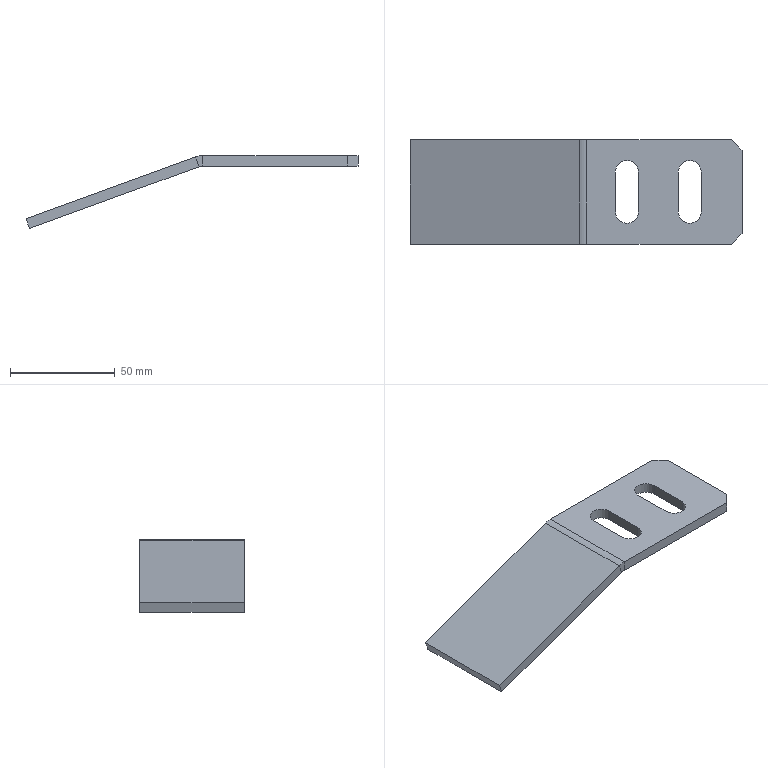Part | SolidWorks | features Chamfer 1, FlatPattern 1, ICE 1, SMBaseFlange 1, SheetMetal 1 | 1 solid | 24 faces | box 158.693 x 50 x 34.796 mm | volume 37608 mm3 | plane 18 | cylinder 6 | commonest cylinder face diameters 11 x4 10 x1 20 x1
STEP:
#1=CARTESIAN_POINT('',(-77.657,50.,-0.6031));
#2=VERTEX_POINT('',#1);
#3=CARTESIAN_POINT('',(-75.947,50.,-5.302));
#4=VERTEX_POINT('',#3);
#5=CARTESIAN_POINT('',(-77.657,50.,-0.6031));
#6=DIRECTION('',(0.342,0.,-0.9397));
#7=VECTOR('',#6,1000.);
#8=LINE('',#5,#7);
#9=EDGE_CURVE('',#2,#4,#8,.T.);
#10=ORIENTED_EDGE('',*,*,#9,.F.);
#11=CARTESIAN_POINT('',(-74.237,50.,0.));
#12=VERTEX_POINT('',#11);
#13=CARTESIAN_POINT('',(-74.237,50.,-10.));
#14=DIRECTION('',(0.,-1.,0.));
#15=DIRECTION('',(0.,0.,1.));
#16=AXIS2_PLACEMENT_3D('',#13,#14,#15);
#17=CIRCLE('',#16,10.);
#18=EDGE_CURVE('',#12,#2,#17,.T.);
#19=ORIENTED_EDGE('',*,*,#18,.F.);
#20=CARTESIAN_POINT('',(-74.237,50.,-5.));
#21=VERTEX_POINT('',#20);
#22=CARTESIAN_POINT('',(-74.237,50.,-5.));
#23=DIRECTION('',(0.,0.,1.));
#24=VECTOR('',#23,1000.);
#25=LINE('',#22,#24);
#26=EDGE_CURVE('',#21,#12,#25,.T.);
#27=ORIENTED_EDGE('',*,*,#26,.F.);
#28=CARTESIAN_POINT('',(-74.237,50.,-10.));
#29=DIRECTION('',(0.,-1.,0.));
#30=DIRECTION('',(1.,0.,0.));
#31=AXIS2_PLACEMENT_3D('',#28,#29,#30);
#32=CIRCLE('',#31,5.);
#33=EDGE_CURVE('',#21,#4,#32,.T.);
#34=ORIENTED_EDGE('',*,*,#33,.T.);
#35=EDGE_LOOP('',(#10,#19,#27,#34));
#36=FACE_OUTER_BOUND('',#35,.T.);
#37=CARTESIAN_POINT('',(-77.657,50.,-0.6031));
#38=DIRECTION('',(0.,1.,0.));
#39=DIRECTION('',(0.,0.,1.));
#40=AXIS2_PLACEMENT_3D('',#37,#38,#39);
#41=PLANE('',#40);
#42=ADVANCED_FACE('',(#36),#41,.T.);
#43=CARTESIAN_POINT('',(-158.693,50.,-30.098));
#44=VERTEX_POINT('',#43);
#45=CARTESIAN_POINT('',(-76.,50.,0.));
#46=DIRECTION('',(-0.9397,0.,-0.342));
#47=VECTOR('',#46,1000.);
#48=LINE('',#45,#47);
#49=EDGE_CURVE('',#2,#44,#48,.T.);
#50=ORIENTED_EDGE('',*,*,#49,.F.);
#51=ORIENTED_EDGE('',*,*,#9,.T.);
#52=CARTESIAN_POINT('',(-156.983,50.,-34.796));
#53=VERTEX_POINT('',#52);
#54=CARTESIAN_POINT('',(-74.29,50.,-4.698));
#55=DIRECTION('',(-0.9397,0.,-0.342));
#56=VECTOR('',#55,1000.);
#57=LINE('',#54,#56);
#58=EDGE_CURVE('',#4,#53,#57,.T.);
#59=ORIENTED_EDGE('',*,*,#58,.T.);
#60=CARTESIAN_POINT('',(-158.693,50.,-30.098));
#61=DIRECTION('',(0.342,0.,-0.9397));
#62=VECTOR('',#61,1000.);
#63=LINE('',#60,#62);
#64=EDGE_CURVE('',#44,#53,#63,.T.);
#65=ORIENTED_EDGE('',*,*,#64,.F.);
#66=EDGE_LOOP('',(#50,#51,#59,#65));
#67=FACE_OUTER_BOUND('',#66,.T.);
#68=CARTESIAN_POINT('',(-74.237,50.,-5.));
#69=DIRECTION('',(0.,1.,0.));
#70=DIRECTION('',(0.,0.,1.));
#71=AXIS2_PLACEMENT_3D('',#68,#69,#70);
#72=PLANE('',#71);
#73=ADVANCED_FACE('',(#67),#72,.T.);
#74=CARTESIAN_POINT('',(-74.237,0.,0.));
#75=VERTEX_POINT('',#74);
#76=CARTESIAN_POINT('',(-74.237,0.,-5.));
#77=VERTEX_POINT('',#76);
#78=CARTESIAN_POINT('',(-74.237,0.,0.));
#79=DIRECTION('',(0.,0.,-1.));
#80=VECTOR('',#79,1000.);
#81=LINE('',#78,#80);
#82=EDGE_CURVE('',#75,#77,#81,.T.);
#83=ORIENTED_EDGE('',*,*,#82,.F.);
#84=CARTESIAN_POINT('',(-77.657,0.,-0.6031));
#85=VERTEX_POINT('',#84);
#86=CARTESIAN_POINT('',(-74.237,0.,-10.));
#87=DIRECTION('',(0.,-1.,0.));
#88=DIRECTION('',(0.,0.,1.));
#89=AXIS2_PLACEMENT_3D('',#86,#87,#88);
#90=CIRCLE('',#89,10.);
#91=EDGE_CURVE('',#75,#85,#90,.T.);
#92=ORIENTED_EDGE('',*,*,#91,.T.);
#93=CARTESIAN_POINT('',(-75.947,0.,-5.302));
#94=VERTEX_POINT('',#93);
#95=CARTESIAN_POINT('',(-75.947,0.,-5.302));
#96=DIRECTION('',(-0.342,0.,0.9397));
#97=VECTOR('',#96,1000.);
#98=LINE('',#95,#97);
#99=EDGE_CURVE('',#94,#85,#98,.T.);
#100=ORIENTED_EDGE('',*,*,#99,.F.);
#101=CARTESIAN_POINT('',(-74.237,0.,-10.));
#102=DIRECTION('',(0.,-1.,0.));
#103=DIRECTION('',(1.,0.,0.));
#104=AXIS2_PLACEMENT_3D('',#101,#102,#103);
#105=CIRCLE('',#104,5.);
#106=EDGE_CURVE('',#77,#94,#105,.T.);
#107=ORIENTED_EDGE('',*,*,#106,.F.);
#108=EDGE_LOOP('',(#83,#92,#100,#107));
#109=FACE_OUTER_BOUND('',#108,.T.);
#110=CARTESIAN_POINT('',(-74.237,0.,0.));
#111=DIRECTION('',(0.,-1.,0.));
#112=DIRECTION('',(0.,0.,-1.));
#113=AXIS2_PLACEMENT_3D('',#110,#111,#112);
#114=PLANE('',#113);
#115=ADVANCED_FACE('',(#109),#114,.T.);
#116=CARTESIAN_POINT('',(-5.,0.,-5.));
#117=VERTEX_POINT('',#116);
#118=CARTESIAN_POINT('',(0.,0.,-5.));
#119=DIRECTION('',(-1.,0.,0.));
#120=VECTOR('',#119,1000.);
#121=LINE('',#118,#120);
#122=EDGE_CURVE('',#117,#77,#121,.T.);
#123=ORIENTED_EDGE('',*,*,#122,.F.);
#124=CARTESIAN_POINT('',(-5.,0.,0.));
#125=VERTEX_POINT('',#124);
#126=CARTESIAN_POINT('',(-5.,0.,-5.302));
#127=DIRECTION('',(0.,0.,1.));
#128=VECTOR('',#127,1000.);
#129=LINE('',#126,#128);
#130=EDGE_CURVE('',#117,#125,#129,.T.);
#131=ORIENTED_EDGE('',*,*,#130,.T.);
#132=CARTESIAN_POINT('',(0.,0.,0.));
#133=DIRECTION('',(-1.,0.,0.));
#134=VECTOR('',#133,1000.);
#135=LINE('',#132,#134);
#136=EDGE_CURVE('',#125,#75,#135,.T.);
#137=ORIENTED_EDGE('',*,*,#136,.T.);
#138=ORIENTED_EDGE('',*,*,#82,.T.);
#139=EDGE_LOOP('',(#123,#131,#137,#138));
#140=FACE_OUTER_BOUND('',#139,.T.);
#141=CARTESIAN_POINT('',(-75.947,0.,-5.302));
#142=DIRECTION('',(0.,-1.,0.));
#143=DIRECTION('',(0.,0.,-1.));
#144=AXIS2_PLACEMENT_3D('',#141,#142,#143);
#145=PLANE('',#144);
#146=ADVANCED_FACE('',(#140),#145,.T.);
#147=CARTESIAN_POINT('',(-156.983,0.,-34.796));
#148=VERTEX_POINT('',#147);
#149=CARTESIAN_POINT('',(-74.29,0.,-4.698));
#150=DIRECTION('',(-0.9397,0.,-0.342));
#151=VECTOR('',#150,1000.);
#152=LINE('',#149,#151);
#153=EDGE_CURVE('',#94,#148,#152,.T.);
#154=ORIENTED_EDGE('',*,*,#153,.T.);
#155=CARTESIAN_POINT('',(-156.983,50.,-34.796));
#156=DIRECTION('',(0.,-1.,0.));
#157=VECTOR('',#156,1000.);
#158=LINE('',#155,#157);
#159=EDGE_CURVE('',#53,#148,#158,.T.);
#160=ORIENTED_EDGE('',*,*,#159,.F.);
#161=ORIENTED_EDGE('',*,*,#58,.F.);
#162=CARTESIAN_POINT('',(-75.947,50.,-5.302));
#163=DIRECTION('',(0.,-1.,0.));
#164=VECTOR('',#163,1000.);
#165=LINE('',#162,#164);
#166=EDGE_CURVE('',#4,#94,#165,.T.);
#167=ORIENTED_EDGE('',*,*,#166,.T.);
#168=EDGE_LOOP('',(#154,#160,#161,#167));
#169=FACE_OUTER_BOUND('',#168,.T.);
#170=CARTESIAN_POINT('',(-74.29,50.,-4.698));
#171=DIRECTION('',(-0.342,0.,0.9397));
#172=DIRECTION('',(0.9397,0.,0.342));
#173=AXIS2_PLACEMENT_3D('',#170,#171,#172);
#174=PLANE('',#173);
#175=ADVANCED_FACE('',(#169),#174,.F.);
#176=CARTESIAN_POINT('',(-158.693,0.,-30.098));
#177=VERTEX_POINT('',#176);
#178=CARTESIAN_POINT('',(-158.693,0.,-30.098));
#179=DIRECTION('',(0.342,0.,-0.9397));
#180=VECTOR('',#179,1000.);
#181=LINE('',#178,#180);
#182=EDGE_CURVE('',#177,#148,#181,.T.);
#183=ORIENTED_EDGE('',*,*,#182,.F.);
#184=CARTESIAN_POINT('',(-158.693,50.,-30.098));
#185=DIRECTION('',(0.,-1.,0.));
#186=VECTOR('',#185,1000.);
#187=LINE('',#184,#186);
#188=EDGE_CURVE('',#44,#177,#187,.T.);
#189=ORIENTED_EDGE('',*,*,#188,.F.);
#190=ORIENTED_EDGE('',*,*,#64,.T.);
#191=ORIENTED_EDGE('',*,*,#159,.T.);
#192=EDGE_LOOP('',(#183,#189,#190,#191));
#193=FACE_OUTER_BOUND('',#192,.T.);
#194=CARTESIAN_POINT('',(-158.693,50.,-30.098));
#195=DIRECTION('',(-0.9397,0.,-0.342));
#196=DIRECTION('',(-0.342,0.,0.9397));
#197=AXIS2_PLACEMENT_3D('',#194,#195,#196);
#198=PLANE('',#197);
#199=ADVANCED_FACE('',(#193),#198,.T.);
#200=CARTESIAN_POINT('',(-76.,0.,0.));
#201=DIRECTION('',(-0.9397,0.,-0.342));
#202=VECTOR('',#201,1000.);
#203=LINE('',#200,#202);
#204=EDGE_CURVE('',#85,#177,#203,.T.);
#205=ORIENTED_EDGE('',*,*,#204,.F.);
#206=CARTESIAN_POINT('',(-77.657,50.,-0.6031));
#207=DIRECTION('',(0.,-1.,0.));
#208=VECTOR('',#207,1000.);
#209=LINE('',#206,#208);
#210=EDGE_CURVE('',#2,#85,#209,.T.);
#211=ORIENTED_EDGE('',*,*,#210,.F.);
#212=ORIENTED_EDGE('',*,*,#49,.T.);
#213=ORIENTED_EDGE('',*,*,#188,.T.);
#214=EDGE_LOOP('',(#205,#211,#212,#213));
#215=FACE_OUTER_BOUND('',#214,.T.);
#216=CARTESIAN_POINT('',(-76.,50.,0.));
#217=DIRECTION('',(-0.342,0.,0.9397));
#218=DIRECTION('',(0.9397,0.,0.342));
#219=AXIS2_PLACEMENT_3D('',#216,#217,#218);
#220=PLANE('',#219);
#221=ADVANCED_FACE('',(#215),#220,.T.);
#222=ORIENTED_EDGE('',*,*,#91,.F.);
#223=CARTESIAN_POINT('',(-74.237,50.,0.));
#224=DIRECTION('',(0.,-1.,0.));
#225=VECTOR('',#224,1000.);
#226=LINE('',#223,#225);
#227=EDGE_CURVE('',#12,#75,#226,.T.);
#228=ORIENTED_EDGE('',*,*,#227,.F.);
#229=ORIENTED_EDGE('',*,*,#18,.T.);
#230=ORIENTED_EDGE('',*,*,#210,.T.);
#231=EDGE_LOOP('',(#222,#228,#229,#230));
#232=FACE_OUTER_BOUND('',#231,.T.);
#233=CARTESIAN_POINT('',(-74.237,50.,-10.));
#234=DIRECTION('',(0.,-1.,0.));
#235=DIRECTION('',(0.,0.,-1.));
#236=AXIS2_PLACEMENT_3D('',#233,#234,#235);
#237=CYLINDRICAL_SURFACE('',#236,10.);
#238=ADVANCED_FACE('',(#232),#237,.T.);
#239=CARTESIAN_POINT('',(-19.5,34.5,0.));
#240=VERTEX_POINT('',#239);
#241=CARTESIAN_POINT('',(-30.5,34.5,0.));
#242=VERTEX_POINT('',#241);
#243=CARTESIAN_POINT('',(-25.,34.5,0.));
#244=DIRECTION('',(0.,0.,1.));
#245=DIRECTION('',(1.,0.,0.));
#246=AXIS2_PLACEMENT_3D('',#243,#244,#245);
#247=CIRCLE('',#246,5.5);
#248=EDGE_CURVE('',#240,#242,#247,.T.);
#249=ORIENTED_EDGE('',*,*,#248,.F.);
#250=CARTESIAN_POINT('',(-19.5,15.5,0.));
#251=VERTEX_POINT('',#250);
#252=CARTESIAN_POINT('',(-19.5,34.5,0.));
#253=DIRECTION('',(0.,1.,0.));
#254=VECTOR('',#253,1000.);
#255=LINE('',#252,#254);
#256=EDGE_CURVE('',#251,#240,#255,.T.);
#257=ORIENTED_EDGE('',*,*,#256,.F.);
#258=CARTESIAN_POINT('',(-30.5,15.5,0.));
#259=VERTEX_POINT('',#258);
#260=CARTESIAN_POINT('',(-25.,15.5,0.));
#261=DIRECTION('',(0.,0.,1.));
#262=DIRECTION('',(1.,0.,0.));
#263=AXIS2_PLACEMENT_3D('',#260,#261,#262);
#264=CIRCLE('',#263,5.5);
#265=EDGE_CURVE('',#259,#251,#264,.T.);
#266=ORIENTED_EDGE('',*,*,#265,.F.);
#267=CARTESIAN_POINT('',(-30.5,34.5,0.));
#268=DIRECTION('',(0.,-1.,0.));
#269=VECTOR('',#268,1000.);
#270=LINE('',#267,#269);
#271=EDGE_CURVE('',#242,#259,#270,.T.);
#272=ORIENTED_EDGE('',*,*,#271,.F.);
#273=EDGE_LOOP('',(#249,#257,#266,#272));
#274=FACE_BOUND('',#273,.T.);
#275=CARTESIAN_POINT('',(-49.5,34.5,0.));
#276=VERTEX_POINT('',#275);
#277=CARTESIAN_POINT('',(-60.5,34.5,0.));
#278=VERTEX_POINT('',#277);
#279=CARTESIAN_POINT('',(-55.,34.5,0.));
#280=DIRECTION('',(0.,0.,1.));
#281=DIRECTION('',(1.,0.,0.));
#282=AXIS2_PLACEMENT_3D('',#279,#280,#281);
#283=CIRCLE('',#282,5.5);
#284=EDGE_CURVE('',#276,#278,#283,.T.);
#285=ORIENTED_EDGE('',*,*,#284,.F.);
#286=CARTESIAN_POINT('',(-49.5,15.5,0.));
#287=VERTEX_POINT('',#286);
#288=CARTESIAN_POINT('',(-49.5,34.5,0.));
#289=DIRECTION('',(0.,1.,0.));
#290=VECTOR('',#289,1000.);
#291=LINE('',#288,#290);
#292=EDGE_CURVE('',#287,#276,#291,.T.);
#293=ORIENTED_EDGE('',*,*,#292,.F.);
#294=CARTESIAN_POINT('',(-60.5,15.5,0.));
#295=VERTEX_POINT('',#294);
#296=CARTESIAN_POINT('',(-55.,15.5,0.));
#297=DIRECTION('',(0.,0.,1.));
#298=DIRECTION('',(1.,0.,0.));
#299=AXIS2_PLACEMENT_3D('',#296,#297,#298);
#300=CIRCLE('',#299,5.5);
#301=EDGE_CURVE('',#295,#287,#300,.T.);
#302=ORIENTED_EDGE('',*,*,#301,.F.);
#303=CARTESIAN_POINT('',(-60.5,34.5,0.));
#304=DIRECTION('',(0.,-1.,0.));
#305=VECTOR('',#304,1000.);
#306=LINE('',#303,#305);
#307=EDGE_CURVE('',#278,#295,#306,.T.);
#308=ORIENTED_EDGE('',*,*,#307,.F.);
#309=EDGE_LOOP('',(#285,#293,#302,#308));
#310=FACE_BOUND('',#309,.T.);
#311=ORIENTED_EDGE('',*,*,#136,.F.);
#312=CARTESIAN_POINT('',(0.,5.,0.));
#313=VERTEX_POINT('',#312);
#314=CARTESIAN_POINT('',(22.5,27.5,0.));
#315=DIRECTION('',(0.7071,0.7071,0.));
#316=VECTOR('',#315,1000.);
#317=LINE('',#314,#316);
#318=EDGE_CURVE('',#125,#313,#317,.T.);
#319=ORIENTED_EDGE('',*,*,#318,.T.);
#320=CARTESIAN_POINT('',(0.,45.,0.));
#321=VERTEX_POINT('',#320);
#322=CARTESIAN_POINT('',(0.,50.,0.));
#323=DIRECTION('',(0.,-1.,0.));
#324=VECTOR('',#323,1000.);
#325=LINE('',#322,#324);
#326=EDGE_CURVE('',#321,#313,#325,.T.);
#327=ORIENTED_EDGE('',*,*,#326,.F.);
#328=CARTESIAN_POINT('',(-5.,50.,0.));
#329=VERTEX_POINT('',#328);
#330=CARTESIAN_POINT('',(-2.5,47.5,0.));
#331=DIRECTION('',(-0.7071,0.7071,0.));
#332=VECTOR('',#331,1000.);
#333=LINE('',#330,#332);
#334=EDGE_CURVE('',#321,#329,#333,.T.);
#335=ORIENTED_EDGE('',*,*,#334,.T.);
#336=CARTESIAN_POINT('',(0.,50.,0.));
#337=DIRECTION('',(-1.,0.,0.));
#338=VECTOR('',#337,1000.);
#339=LINE('',#336,#338);
#340=EDGE_CURVE('',#329,#12,#339,.T.);
#341=ORIENTED_EDGE('',*,*,#340,.T.);
#342=ORIENTED_EDGE('',*,*,#227,.T.);
#343=EDGE_LOOP('',(#311,#319,#327,#335,#341,#342));
#344=FACE_OUTER_BOUND('',#343,.T.);
#345=CARTESIAN_POINT('',(0.,50.,0.));
#346=DIRECTION('',(0.,0.,1.));
#347=DIRECTION('',(1.,0.,0.));
#348=AXIS2_PLACEMENT_3D('',#345,#346,#347);
#349=PLANE('',#348);
#350=ADVANCED_FACE('',(#274,#310,#344),#349,.T.);
#351=ORIENTED_EDGE('',*,*,#326,.T.);
#352=CARTESIAN_POINT('',(0.,5.,-5.));
#353=VERTEX_POINT('',#352);
#354=CARTESIAN_POINT('',(0.,5.,-5.));
#355=DIRECTION('',(0.,0.,-1.));
#356=VECTOR('',#355,1000.);
#357=LINE('',#354,#356);
#358=EDGE_CURVE('',#313,#353,#357,.T.);
#359=ORIENTED_EDGE('',*,*,#358,.T.);
#360=CARTESIAN_POINT('',(0.,45.,-5.));
#361=VERTEX_POINT('',#360);
#362=CARTESIAN_POINT('',(0.,50.,-5.));
#363=DIRECTION('',(0.,-1.,0.));
#364=VECTOR('',#363,1000.);
#365=LINE('',#362,#364);
#366=EDGE_CURVE('',#361,#353,#365,.T.);
#367=ORIENTED_EDGE('',*,*,#366,.F.);
#368=CARTESIAN_POINT('',(0.,45.,-5.));
#369=DIRECTION('',(0.,0.,1.));
#370=VECTOR('',#369,1000.);
#371=LINE('',#368,#370);
#372=EDGE_CURVE('',#361,#321,#371,.T.);
#373=ORIENTED_EDGE('',*,*,#372,.T.);
#374=EDGE_LOOP('',(#351,#359,#367,#373));
#375=FACE_OUTER_BOUND('',#374,.T.);
#376=CARTESIAN_POINT('',(0.,50.,-5.));
#377=DIRECTION('',(1.,0.,0.));
#378=DIRECTION('',(0.,0.,-1.));
#379=AXIS2_PLACEMENT_3D('',#376,#377,#378);
#380=PLANE('',#379);
#381=ADVANCED_FACE('',(#375),#380,.T.);
#382=CARTESIAN_POINT('',(-19.5,15.5,-5.));
#383=VERTEX_POINT('',#382);
#384=CARTESIAN_POINT('',(-19.5,34.5,-5.));
#385=VERTEX_POINT('',#384);
#386=CARTESIAN_POINT('',(-19.5,50.,-5.));
#387=DIRECTION('',(0.,1.,0.));
#388=VECTOR('',#387,1000.);
#389=LINE('',#386,#388);
#390=EDGE_CURVE('',#383,#385,#389,.T.);
#391=ORIENTED_EDGE('',*,*,#390,.T.);
#392=CARTESIAN_POINT('',(-30.5,34.5,-5.));
#393=VERTEX_POINT('',#392);
#394=CARTESIAN_POINT('',(-25.,34.5,-5.));
#395=DIRECTION('',(0.,0.,1.));
#396=DIRECTION('',(1.,0.,0.));
#397=AXIS2_PLACEMENT_3D('',#394,#395,#396);
#398=CIRCLE('',#397,5.5);
#399=EDGE_CURVE('',#385,#393,#398,.T.);
#400=ORIENTED_EDGE('',*,*,#399,.T.);
#401=CARTESIAN_POINT('',(-30.5,15.5,-5.));
#402=VERTEX_POINT('',#401);
#403=CARTESIAN_POINT('',(-30.5,50.,-5.));
#404=DIRECTION('',(0.,-1.,0.));
#405=VECTOR('',#404,1000.);
#406=LINE('',#403,#405);
#407=EDGE_CURVE('',#393,#402,#406,.T.);
#408=ORIENTED_EDGE('',*,*,#407,.T.);
#409=CARTESIAN_POINT('',(-25.,15.5,-5.));
#410=DIRECTION('',(0.,0.,1.));
#411=DIRECTION('',(1.,0.,0.));
#412=AXIS2_PLACEMENT_3D('',#409,#410,#411);
#413=CIRCLE('',#412,5.5);
#414=EDGE_CURVE('',#402,#383,#413,.T.);
#415=ORIENTED_EDGE('',*,*,#414,.T.);
#416=EDGE_LOOP('',(#391,#400,#408,#415));
#417=FACE_BOUND('',#416,.T.);
#418=CARTESIAN_POINT('',(-49.5,15.5,-5.));
#419=VERTEX_POINT('',#418);
#420=CARTESIAN_POINT('',(-49.5,34.5,-5.));
#421=VERTEX_POINT('',#420);
#422=CARTESIAN_POINT('',(-49.5,50.,-5.));
#423=DIRECTION('',(0.,1.,0.));
#424=VECTOR('',#423,1000.);
#425=LINE('',#422,#424);
#426=EDGE_CURVE('',#419,#421,#425,.T.);
#427=ORIENTED_EDGE('',*,*,#426,.T.);
#428=CARTESIAN_POINT('',(-60.5,34.5,-5.));
#429=VERTEX_POINT('',#428);
#430=CARTESIAN_POINT('',(-55.,34.5,-5.));
#431=DIRECTION('',(0.,0.,1.));
#432=DIRECTION('',(1.,0.,0.));
#433=AXIS2_PLACEMENT_3D('',#430,#431,#432);
#434=CIRCLE('',#433,5.5);
#435=EDGE_CURVE('',#421,#429,#434,.T.);
#436=ORIENTED_EDGE('',*,*,#435,.T.);
#437=CARTESIAN_POINT('',(-60.5,15.5,-5.));
#438=VERTEX_POINT('',#437);
#439=CARTESIAN_POINT('',(-60.5,50.,-5.));
#440=DIRECTION('',(0.,-1.,0.));
#441=VECTOR('',#440,1000.);
#442=LINE('',#439,#441);
#443=EDGE_CURVE('',#429,#438,#442,.T.);
#444=ORIENTED_EDGE('',*,*,#443,.T.);
#445=CARTESIAN_POINT('',(-55.,15.5,-5.));
#446=DIRECTION('',(0.,0.,1.));
#447=DIRECTION('',(1.,0.,0.));
#448=AXIS2_PLACEMENT_3D('',#445,#446,#447);
#449=CIRCLE('',#448,5.5);
#450=EDGE_CURVE('',#438,#419,#449,.T.);
#451=ORIENTED_EDGE('',*,*,#450,.T.);
#452=EDGE_LOOP('',(#427,#436,#444,#451));
#453=FACE_BOUND('',#452,.T.);
#454=ORIENTED_EDGE('',*,*,#366,.T.);
#455=CARTESIAN_POINT('',(-5.,0.,-5.));
#456=DIRECTION('',(-0.7071,-0.7071,0.));
#457=VECTOR('',#456,1000.);
#458=LINE('',#455,#457);
#459=EDGE_CURVE('',#353,#117,#458,.T.);
#460=ORIENTED_EDGE('',*,*,#459,.T.);
#461=ORIENTED_EDGE('',*,*,#122,.T.);
#462=CARTESIAN_POINT('',(-74.237,50.,-5.));
#463=DIRECTION('',(0.,-1.,0.));
#464=VECTOR('',#463,1000.);
#465=LINE('',#462,#464);
#466=EDGE_CURVE('',#21,#77,#465,.T.);
#467=ORIENTED_EDGE('',*,*,#466,.F.);
#468=CARTESIAN_POINT('',(-5.,50.,-5.));
#469=VERTEX_POINT('',#468);
#470=CARTESIAN_POINT('',(0.,50.,-5.));
#471=DIRECTION('',(-1.,0.,0.));
#472=VECTOR('',#471,1000.);
#473=LINE('',#470,#472);
#474=EDGE_CURVE('',#469,#21,#473,.T.);
#475=ORIENTED_EDGE('',*,*,#474,.F.);
#476=CARTESIAN_POINT('',(0.,45.,-5.));
#477=DIRECTION('',(0.7071,-0.7071,0.));
#478=VECTOR('',#477,1000.);
#479=LINE('',#476,#478);
#480=EDGE_CURVE('',#469,#361,#479,.T.);
#481=ORIENTED_EDGE('',*,*,#480,.T.);
#482=EDGE_LOOP('',(#454,#460,#461,#467,#475,#481));
#483=FACE_OUTER_BOUND('',#482,.T.);
#484=CARTESIAN_POINT('',(0.,50.,-5.));
#485=DIRECTION('',(0.,0.,1.));
#486=DIRECTION('',(1.,0.,0.));
#487=AXIS2_PLACEMENT_3D('',#484,#485,#486);
#488=PLANE('',#487);
#489=ADVANCED_FACE('',(#417,#453,#483),#488,.F.);
#490=ORIENTED_EDGE('',*,*,#106,.T.);
#491=ORIENTED_EDGE('',*,*,#166,.F.);
#492=ORIENTED_EDGE('',*,*,#33,.F.);
#493=ORIENTED_EDGE('',*,*,#466,.T.);
#494=EDGE_LOOP('',(#490,#491,#492,#493));
#495=FACE_OUTER_BOUND('',#494,.T.);
#496=CARTESIAN_POINT('',(-74.237,50.,-10.));
#497=DIRECTION('',(0.,-1.,0.));
#498=DIRECTION('',(0.,0.,-1.));
#499=AXIS2_PLACEMENT_3D('',#496,#497,#498);
#500=CYLINDRICAL_SURFACE('',#499,5.);
#501=ADVANCED_FACE('',(#495),#500,.F.);
#502=ORIENTED_EDGE('',*,*,#340,.F.);
#503=CARTESIAN_POINT('',(-5.,50.,-10.));
#504=DIRECTION('',(0.,0.,-1.));
#505=VECTOR('',#504,1000.);
#506=LINE('',#503,#505);
#507=EDGE_CURVE('',#329,#469,#506,.T.);
#508=ORIENTED_EDGE('',*,*,#507,.T.);
#509=ORIENTED_EDGE('',*,*,#474,.T.);
#510=ORIENTED_EDGE('',*,*,#26,.T.);
#511=EDGE_LOOP('',(#502,#508,#509,#510));
#512=FACE_OUTER_BOUND('',#511,.T.);
#513=CARTESIAN_POINT('',(-74.237,50.,-10.));
#514=DIRECTION('',(0.,1.,0.));
#515=DIRECTION('',(1.,0.,0.));
#516=AXIS2_PLACEMENT_3D('',#513,#514,#515);
#517=PLANE('',#516);
#518=ADVANCED_FACE('',(#512),#517,.T.);
#519=ORIENTED_EDGE('',*,*,#153,.F.);
#520=ORIENTED_EDGE('',*,*,#99,.T.);
#521=ORIENTED_EDGE('',*,*,#204,.T.);
#522=ORIENTED_EDGE('',*,*,#182,.T.);
#523=EDGE_LOOP('',(#519,#520,#521,#522));
#524=FACE_OUTER_BOUND('',#523,.T.);
#525=CARTESIAN_POINT('',(-74.237,0.,-10.));
#526=DIRECTION('',(0.,1.,0.));
#527=DIRECTION('',(1.,0.,0.));
#528=AXIS2_PLACEMENT_3D('',#525,#526,#527);
#529=PLANE('',#528);
#530=ADVANCED_FACE('',(#524),#529,.F.);
#531=CARTESIAN_POINT('',(-49.5,34.5,-10.));
#532=DIRECTION('',(0.,0.,1.));
#533=VECTOR('',#532,1000.);
#534=LINE('',#531,#533);
#535=EDGE_CURVE('',#421,#276,#534,.T.);
#536=ORIENTED_EDGE('',*,*,#535,.T.);
#537=ORIENTED_EDGE('',*,*,#284,.T.);
#538=CARTESIAN_POINT('',(-60.5,34.5,-10.));
#539=DIRECTION('',(0.,0.,1.));
#540=VECTOR('',#539,1000.);
#541=LINE('',#538,#540);
#542=EDGE_CURVE('',#429,#278,#541,.T.);
#543=ORIENTED_EDGE('',*,*,#542,.F.);
#544=ORIENTED_EDGE('',*,*,#435,.F.);
#545=EDGE_LOOP('',(#536,#537,#543,#544));
#546=FACE_OUTER_BOUND('',#545,.T.);
#547=CARTESIAN_POINT('',(-55.,34.5,-10.));
#548=DIRECTION('',(0.,0.,1.));
#549=DIRECTION('',(1.,0.,0.));
#550=AXIS2_PLACEMENT_3D('',#547,#548,#549);
#551=CYLINDRICAL_SURFACE('',#550,5.5);
#552=ADVANCED_FACE('',(#546),#551,.F.);
#553=CARTESIAN_POINT('',(-49.5,15.5,-10.));
#554=DIRECTION('',(0.,0.,1.));
#555=VECTOR('',#554,1000.);
#556=LINE('',#553,#555);
#557=EDGE_CURVE('',#419,#287,#556,.T.);
#558=ORIENTED_EDGE('',*,*,#557,.T.);
#559=ORIENTED_EDGE('',*,*,#292,.T.);
#560=ORIENTED_EDGE('',*,*,#535,.F.);
#561=ORIENTED_EDGE('',*,*,#426,.F.);
#562=EDGE_LOOP('',(#558,#559,#560,#561));
#563=FACE_OUTER_BOUND('',#562,.T.);
#564=CARTESIAN_POINT('',(-49.5,34.5,-10.));
#565=DIRECTION('',(1.,0.,0.));
#566=DIRECTION('',(0.,0.,-1.));
#567=AXIS2_PLACEMENT_3D('',#564,#565,#566);
#568=PLANE('',#567);
#569=ADVANCED_FACE('',(#563),#568,.F.);
#570=CARTESIAN_POINT('',(-60.5,15.5,-10.));
#571=DIRECTION('',(0.,0.,1.));
#572=VECTOR('',#571,1000.);
#573=LINE('',#570,#572);
#574=EDGE_CURVE('',#438,#295,#573,.T.);
#575=ORIENTED_EDGE('',*,*,#574,.T.);
#576=ORIENTED_EDGE('',*,*,#301,.T.);
#577=ORIENTED_EDGE('',*,*,#557,.F.);
#578=ORIENTED_EDGE('',*,*,#450,.F.);
#579=EDGE_LOOP('',(#575,#576,#577,#578));
#580=FACE_OUTER_BOUND('',#579,.T.);
#581=CARTESIAN_POINT('',(-55.,15.5,-10.));
#582=DIRECTION('',(0.,0.,1.));
#583=DIRECTION('',(1.,0.,0.));
#584=AXIS2_PLACEMENT_3D('',#581,#582,#583);
#585=CYLINDRICAL_SURFACE('',#584,5.5);
#586=ADVANCED_FACE('',(#580),#585,.F.);
#587=ORIENTED_EDGE('',*,*,#542,.T.);
#588=ORIENTED_EDGE('',*,*,#307,.T.);
#589=ORIENTED_EDGE('',*,*,#574,.F.);
#590=ORIENTED_EDGE('',*,*,#443,.F.);
#591=EDGE_LOOP('',(#587,#588,#589,#590));
#592=FACE_OUTER_BOUND('',#591,.T.);
#593=CARTESIAN_POINT('',(-60.5,34.5,-10.));
#594=DIRECTION('',(-1.,0.,0.));
#595=DIRECTION('',(0.,0.,1.));
#596=AXIS2_PLACEMENT_3D('',#593,#594,#595);
#597=PLANE('',#596);
#598=ADVANCED_FACE('',(#592),#597,.F.);
#599=CARTESIAN_POINT('',(-19.5,34.5,-10.));
#600=DIRECTION('',(0.,0.,1.));
#601=VECTOR('',#600,1000.);
#602=LINE('',#599,#601);
#603=EDGE_CURVE('',#385,#240,#602,.T.);
#604=ORIENTED_EDGE('',*,*,#603,.T.);
#605=ORIENTED_EDGE('',*,*,#248,.T.);
#606=CARTESIAN_POINT('',(-30.5,34.5,-10.));
#607=DIRECTION('',(0.,0.,1.));
#608=VECTOR('',#607,1000.);
#609=LINE('',#606,#608);
#610=EDGE_CURVE('',#393,#242,#609,.T.);
#611=ORIENTED_EDGE('',*,*,#610,.F.);
#612=ORIENTED_EDGE('',*,*,#399,.F.);
#613=EDGE_LOOP('',(#604,#605,#611,#612));
#614=FACE_OUTER_BOUND('',#613,.T.);
#615=CARTESIAN_POINT('',(-25.,34.5,-10.));
#616=DIRECTION('',(0.,0.,1.));
#617=DIRECTION('',(1.,0.,0.));
#618=AXIS2_PLACEMENT_3D('',#615,#616,#617);
#619=CYLINDRICAL_SURFACE('',#618,5.5);
#620=ADVANCED_FACE('',(#614),#619,.F.);
#621=CARTESIAN_POINT('',(-19.5,15.5,-10.));
#622=DIRECTION('',(0.,0.,1.));
#623=VECTOR('',#622,1000.);
#624=LINE('',#621,#623);
#625=EDGE_CURVE('',#383,#251,#624,.T.);
#626=ORIENTED_EDGE('',*,*,#625,.T.);
#627=ORIENTED_EDGE('',*,*,#256,.T.);
#628=ORIENTED_EDGE('',*,*,#603,.F.);
#629=ORIENTED_EDGE('',*,*,#390,.F.);
#630=EDGE_LOOP('',(#626,#627,#628,#629));
#631=FACE_OUTER_BOUND('',#630,.T.);
#632=CARTESIAN_POINT('',(-19.5,34.5,-10.));
#633=DIRECTION('',(1.,0.,0.));
#634=DIRECTION('',(0.,0.,-1.));
#635=AXIS2_PLACEMENT_3D('',#632,#633,#634);
#636=PLANE('',#635);
#637=ADVANCED_FACE('',(#631),#636,.F.);
#638=CARTESIAN_POINT('',(-30.5,15.5,-10.));
#639=DIRECTION('',(0.,0.,1.));
#640=VECTOR('',#639,1000.);
#641=LINE('',#638,#640);
#642=EDGE_CURVE('',#402,#259,#641,.T.);
#643=ORIENTED_EDGE('',*,*,#642,.T.);
#644=ORIENTED_EDGE('',*,*,#265,.T.);
#645=ORIENTED_EDGE('',*,*,#625,.F.);
#646=ORIENTED_EDGE('',*,*,#414,.F.);
#647=EDGE_LOOP('',(#643,#644,#645,#646));
#648=FACE_OUTER_BOUND('',#647,.T.);
#649=CARTESIAN_POINT('',(-25.,15.5,-10.));
#650=DIRECTION('',(0.,0.,1.));
#651=DIRECTION('',(1.,0.,0.));
#652=AXIS2_PLACEMENT_3D('',#649,#650,#651);
#653=CYLINDRICAL_SURFACE('',#652,5.5);
#654=ADVANCED_FACE('',(#648),#653,.F.);
#655=ORIENTED_EDGE('',*,*,#610,.T.);
#656=ORIENTED_EDGE('',*,*,#271,.T.);
#657=ORIENTED_EDGE('',*,*,#642,.F.);
#658=ORIENTED_EDGE('',*,*,#407,.F.);
#659=EDGE_LOOP('',(#655,#656,#657,#658));
#660=FACE_OUTER_BOUND('',#659,.T.);
#661=CARTESIAN_POINT('',(-30.5,34.5,-10.));
#662=DIRECTION('',(-1.,0.,0.));
#663=DIRECTION('',(0.,0.,1.));
#664=AXIS2_PLACEMENT_3D('',#661,#662,#663);
#665=PLANE('',#664);
#666=ADVANCED_FACE('',(#660),#665,.F.);
#667=ORIENTED_EDGE('',*,*,#459,.F.);
#668=ORIENTED_EDGE('',*,*,#358,.F.);
#669=ORIENTED_EDGE('',*,*,#318,.F.);
#670=ORIENTED_EDGE('',*,*,#130,.F.);
#671=EDGE_LOOP('',(#667,#668,#669,#670));
#672=FACE_OUTER_BOUND('',#671,.T.);
#673=CARTESIAN_POINT('',(-5.,0.,-5.302));
#674=DIRECTION('',(-0.7071,0.7071,0.));
#675=DIRECTION('',(0.,0.,1.));
#676=AXIS2_PLACEMENT_3D('',#673,#674,#675);
#677=PLANE('',#676);
#678=ADVANCED_FACE('',(#672),#677,.F.);
#679=ORIENTED_EDGE('',*,*,#480,.F.);
#680=ORIENTED_EDGE('',*,*,#507,.F.);
#681=ORIENTED_EDGE('',*,*,#334,.F.);
#682=ORIENTED_EDGE('',*,*,#372,.F.);
#683=EDGE_LOOP('',(#679,#680,#681,#682));
#684=FACE_OUTER_BOUND('',#683,.T.);
#685=CARTESIAN_POINT('',(0.,45.,-5.));
#686=DIRECTION('',(-0.7071,-0.7071,0.));
#687=DIRECTION('',(0.,0.,1.));
#688=AXIS2_PLACEMENT_3D('',#685,#686,#687);
#689=PLANE('',#688);
#690=ADVANCED_FACE('',(#684),#689,.F.);
#691=CLOSED_SHELL('',(#42,#73,#115,#146,#175,#199,#221,#238,#350,#381,#489,#501,#518,#530,#552,#569,#586,#598,#620,#637,#654,#666,#678,#690));
#692=MANIFOLD_SOLID_BREP('',#691);
#693=CARTESIAN_POINT('',(0.,0.,0.));
#694=DIRECTION('',(0.,0.,1.));
#695=DIRECTION('',(1.,0.,0.));
#696=AXIS2_PLACEMENT_3D('',#693,#694,#695);
#697=(LENGTH_UNIT()NAMED_UNIT(*)SI_UNIT(.MILLI.,.METRE.));
#698=UNCERTAINTY_MEASURE_WITH_UNIT(LENGTH_MEASURE(0.00001),#697,'','');
#699=(NAMED_UNIT(*)PLANE_ANGLE_UNIT()SI_UNIT($,.RADIAN.));
#700=(NAMED_UNIT(*)SI_UNIT($,.STERADIAN.)SOLID_ANGLE_UNIT());
#701=(GEOMETRIC_REPRESENTATION_CONTEXT(3)GLOBAL_UNCERTAINTY_ASSIGNED_CONTEXT((#698))GLOBAL_UNIT_ASSIGNED_CONTEXT((#697,#699,#700))REPRESENTATION_CONTEXT('',''));
#702=ADVANCED_BREP_SHAPE_REPRESENTATION('',(#692,#696),#701);